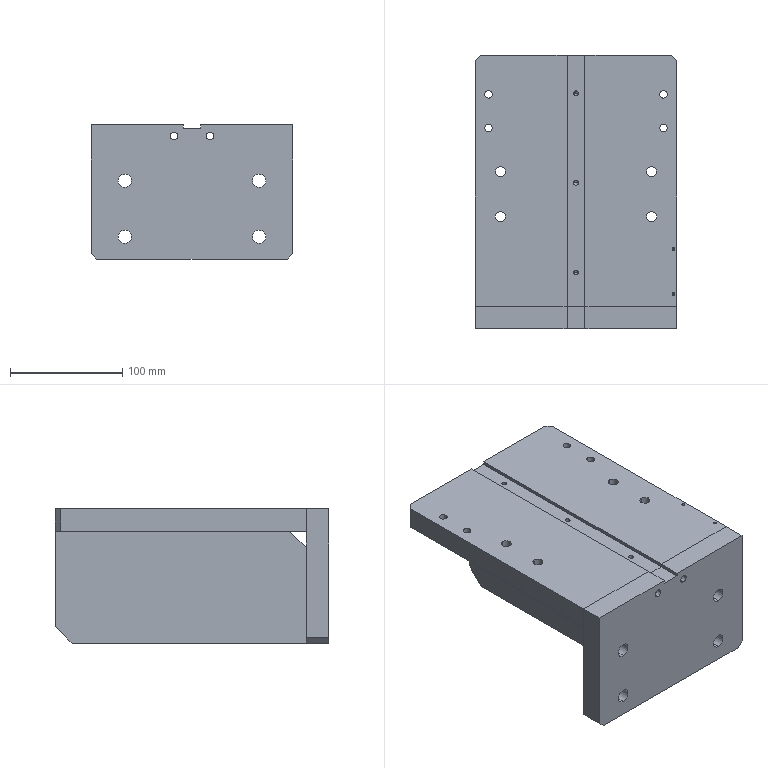Part | STEP file | PN_0008 BKT_Default | 2 solids | 82 faces | box 180 x 244 x 120 mm | volume 1633565 mm3 | cylinder 42 | plane 30 | cone 10 | commonest cylinder face diameters 6.8 x16 9 x8 12 x8 4.2 x6 2.5 x4